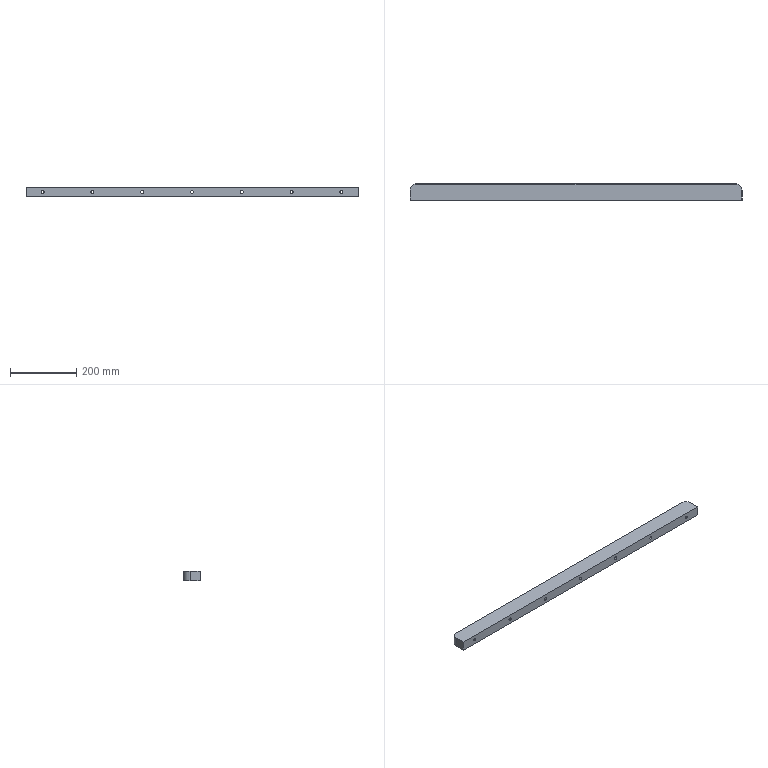Part | STEP file | TJ-DHQM-003-009 | 1 solid | 53 faces | box 1000 x 50 x 30 mm | volume 1451710 mm3 | cylinder 30 | plane 19 | cone 4 | commonest cylinder face diameters 9 x14 15 x14 40 x2
STEP:
#1=CARTESIAN_POINT('',(450.,25.,-7.5));
#2=VERTEX_POINT('',#1);
#3=CARTESIAN_POINT('',(450.,25.,7.5));
#4=VERTEX_POINT('',#3);
#5=CARTESIAN_POINT('',(450.,25.,0.));
#6=DIRECTION('',(0.,1.,0.));
#7=DIRECTION('',(0.,0.,1.));
#8=AXIS2_PLACEMENT_3D('',#5,#6,#7);
#9=CIRCLE('',#8,7.5);
#10=EDGE_CURVE('',#2,#4,#9,.T.);
#11=ORIENTED_EDGE('',*,*,#10,.F.);
#12=CARTESIAN_POINT('',(450.,50.,-7.5));
#13=VERTEX_POINT('',#12);
#14=CARTESIAN_POINT('',(450.,50.,-7.5));
#15=DIRECTION('',(0.,1.,0.));
#16=VECTOR('',#15,1000.);
#17=LINE('',#14,#16);
#18=EDGE_CURVE('',#2,#13,#17,.T.);
#19=ORIENTED_EDGE('',*,*,#18,.T.);
#20=CARTESIAN_POINT('',(450.,50.,7.5));
#21=VERTEX_POINT('',#20);
#22=CARTESIAN_POINT('',(450.,50.,0.));
#23=DIRECTION('',(0.,1.,0.));
#24=DIRECTION('',(0.,0.,1.));
#25=AXIS2_PLACEMENT_3D('',#22,#23,#24);
#26=CIRCLE('',#25,7.5);
#27=EDGE_CURVE('',#13,#21,#26,.T.);
#28=ORIENTED_EDGE('',*,*,#27,.T.);
#29=CARTESIAN_POINT('',(450.,50.,7.5));
#30=DIRECTION('',(0.,1.,0.));
#31=VECTOR('',#30,1000.);
#32=LINE('',#29,#31);
#33=EDGE_CURVE('',#4,#21,#32,.T.);
#34=ORIENTED_EDGE('',*,*,#33,.F.);
#35=EDGE_LOOP('',(#11,#19,#28,#34));
#36=FACE_OUTER_BOUND('',#35,.T.);
#37=CARTESIAN_POINT('',(450.,50.,0.));
#38=DIRECTION('',(0.,1.,0.));
#39=DIRECTION('',(0.,0.,1.));
#40=AXIS2_PLACEMENT_3D('',#37,#38,#39);
#41=CYLINDRICAL_SURFACE('',#40,7.5);
#42=ADVANCED_FACE('',(#36),#41,.F.);
#43=CARTESIAN_POINT('',(450.,0.,-4.5));
#44=VERTEX_POINT('',#43);
#45=CARTESIAN_POINT('',(450.,0.,4.5));
#46=VERTEX_POINT('',#45);
#47=CARTESIAN_POINT('',(450.,0.,0.));
#48=DIRECTION('',(0.,1.,0.));
#49=DIRECTION('',(0.,0.,1.));
#50=AXIS2_PLACEMENT_3D('',#47,#48,#49);
#51=CIRCLE('',#50,4.5);
#52=EDGE_CURVE('',#44,#46,#51,.T.);
#53=ORIENTED_EDGE('',*,*,#52,.F.);
#54=CARTESIAN_POINT('',(450.,25.,-4.5));
#55=VERTEX_POINT('',#54);
#56=CARTESIAN_POINT('',(450.,50.,-4.5));
#57=DIRECTION('',(0.,1.,0.));
#58=VECTOR('',#57,1000.);
#59=LINE('',#56,#58);
#60=EDGE_CURVE('',#44,#55,#59,.T.);
#61=ORIENTED_EDGE('',*,*,#60,.T.);
#62=CARTESIAN_POINT('',(450.,25.,4.5));
#63=VERTEX_POINT('',#62);
#64=CARTESIAN_POINT('',(450.,25.,0.));
#65=DIRECTION('',(0.,1.,0.));
#66=DIRECTION('',(0.,0.,1.));
#67=AXIS2_PLACEMENT_3D('',#64,#65,#66);
#68=CIRCLE('',#67,4.5);
#69=EDGE_CURVE('',#55,#63,#68,.T.);
#70=ORIENTED_EDGE('',*,*,#69,.T.);
#71=CARTESIAN_POINT('',(450.,50.,4.5));
#72=DIRECTION('',(0.,1.,0.));
#73=VECTOR('',#72,1000.);
#74=LINE('',#71,#73);
#75=EDGE_CURVE('',#46,#63,#74,.T.);
#76=ORIENTED_EDGE('',*,*,#75,.F.);
#77=EDGE_LOOP('',(#53,#61,#70,#76));
#78=FACE_OUTER_BOUND('',#77,.T.);
#79=CARTESIAN_POINT('',(450.,50.,0.));
#80=DIRECTION('',(0.,1.,0.));
#81=DIRECTION('',(0.,0.,1.));
#82=AXIS2_PLACEMENT_3D('',#79,#80,#81);
#83=CYLINDRICAL_SURFACE('',#82,4.5);
#84=ADVANCED_FACE('',(#78),#83,.F.);
#85=CARTESIAN_POINT('',(300.,25.,-7.5));
#86=VERTEX_POINT('',#85);
#87=CARTESIAN_POINT('',(300.,25.,7.5));
#88=VERTEX_POINT('',#87);
#89=CARTESIAN_POINT('',(300.,25.,0.));
#90=DIRECTION('',(0.,1.,0.));
#91=DIRECTION('',(0.,0.,1.));
#92=AXIS2_PLACEMENT_3D('',#89,#90,#91);
#93=CIRCLE('',#92,7.5);
#94=EDGE_CURVE('',#86,#88,#93,.T.);
#95=ORIENTED_EDGE('',*,*,#94,.F.);
#96=CARTESIAN_POINT('',(300.,50.,-7.5));
#97=VERTEX_POINT('',#96);
#98=CARTESIAN_POINT('',(300.,50.,-7.5));
#99=DIRECTION('',(0.,1.,0.));
#100=VECTOR('',#99,1000.);
#101=LINE('',#98,#100);
#102=EDGE_CURVE('',#86,#97,#101,.T.);
#103=ORIENTED_EDGE('',*,*,#102,.T.);
#104=CARTESIAN_POINT('',(300.,50.,7.5));
#105=VERTEX_POINT('',#104);
#106=CARTESIAN_POINT('',(300.,50.,0.));
#107=DIRECTION('',(0.,1.,0.));
#108=DIRECTION('',(0.,0.,1.));
#109=AXIS2_PLACEMENT_3D('',#106,#107,#108);
#110=CIRCLE('',#109,7.5);
#111=EDGE_CURVE('',#97,#105,#110,.T.);
#112=ORIENTED_EDGE('',*,*,#111,.T.);
#113=CARTESIAN_POINT('',(300.,50.,7.5));
#114=DIRECTION('',(0.,1.,0.));
#115=VECTOR('',#114,1000.);
#116=LINE('',#113,#115);
#117=EDGE_CURVE('',#88,#105,#116,.T.);
#118=ORIENTED_EDGE('',*,*,#117,.F.);
#119=EDGE_LOOP('',(#95,#103,#112,#118));
#120=FACE_OUTER_BOUND('',#119,.T.);
#121=CARTESIAN_POINT('',(300.,50.,0.));
#122=DIRECTION('',(0.,1.,0.));
#123=DIRECTION('',(0.,0.,1.));
#124=AXIS2_PLACEMENT_3D('',#121,#122,#123);
#125=CYLINDRICAL_SURFACE('',#124,7.5);
#126=ADVANCED_FACE('',(#120),#125,.F.);
#127=CARTESIAN_POINT('',(300.,0.,-4.5));
#128=VERTEX_POINT('',#127);
#129=CARTESIAN_POINT('',(300.,0.,4.5));
#130=VERTEX_POINT('',#129);
#131=CARTESIAN_POINT('',(300.,0.,0.));
#132=DIRECTION('',(0.,1.,0.));
#133=DIRECTION('',(0.,0.,1.));
#134=AXIS2_PLACEMENT_3D('',#131,#132,#133);
#135=CIRCLE('',#134,4.5);
#136=EDGE_CURVE('',#128,#130,#135,.T.);
#137=ORIENTED_EDGE('',*,*,#136,.F.);
#138=CARTESIAN_POINT('',(300.,25.,-4.5));
#139=VERTEX_POINT('',#138);
#140=CARTESIAN_POINT('',(300.,50.,-4.5));
#141=DIRECTION('',(0.,1.,0.));
#142=VECTOR('',#141,1000.);
#143=LINE('',#140,#142);
#144=EDGE_CURVE('',#128,#139,#143,.T.);
#145=ORIENTED_EDGE('',*,*,#144,.T.);
#146=CARTESIAN_POINT('',(300.,25.,4.5));
#147=VERTEX_POINT('',#146);
#148=CARTESIAN_POINT('',(300.,25.,0.));
#149=DIRECTION('',(0.,1.,0.));
#150=DIRECTION('',(0.,0.,1.));
#151=AXIS2_PLACEMENT_3D('',#148,#149,#150);
#152=CIRCLE('',#151,4.5);
#153=EDGE_CURVE('',#139,#147,#152,.T.);
#154=ORIENTED_EDGE('',*,*,#153,.T.);
#155=CARTESIAN_POINT('',(300.,50.,4.5));
#156=DIRECTION('',(0.,1.,0.));
#157=VECTOR('',#156,1000.);
#158=LINE('',#155,#157);
#159=EDGE_CURVE('',#130,#147,#158,.T.);
#160=ORIENTED_EDGE('',*,*,#159,.F.);
#161=EDGE_LOOP('',(#137,#145,#154,#160));
#162=FACE_OUTER_BOUND('',#161,.T.);
#163=CARTESIAN_POINT('',(300.,50.,0.));
#164=DIRECTION('',(0.,1.,0.));
#165=DIRECTION('',(0.,0.,1.));
#166=AXIS2_PLACEMENT_3D('',#163,#164,#165);
#167=CYLINDRICAL_SURFACE('',#166,4.5);
#168=ADVANCED_FACE('',(#162),#167,.F.);
#169=CARTESIAN_POINT('',(150.,25.,-7.5));
#170=VERTEX_POINT('',#169);
#171=CARTESIAN_POINT('',(150.,25.,7.5));
#172=VERTEX_POINT('',#171);
#173=CARTESIAN_POINT('',(150.,25.,0.));
#174=DIRECTION('',(0.,1.,0.));
#175=DIRECTION('',(0.,0.,1.));
#176=AXIS2_PLACEMENT_3D('',#173,#174,#175);
#177=CIRCLE('',#176,7.5);
#178=EDGE_CURVE('',#170,#172,#177,.T.);
#179=ORIENTED_EDGE('',*,*,#178,.F.);
#180=CARTESIAN_POINT('',(150.,50.,-7.5));
#181=VERTEX_POINT('',#180);
#182=CARTESIAN_POINT('',(150.,50.,-7.5));
#183=DIRECTION('',(0.,1.,0.));
#184=VECTOR('',#183,1000.);
#185=LINE('',#182,#184);
#186=EDGE_CURVE('',#170,#181,#185,.T.);
#187=ORIENTED_EDGE('',*,*,#186,.T.);
#188=CARTESIAN_POINT('',(150.,50.,7.5));
#189=VERTEX_POINT('',#188);
#190=CARTESIAN_POINT('',(150.,50.,0.));
#191=DIRECTION('',(0.,1.,0.));
#192=DIRECTION('',(0.,0.,1.));
#193=AXIS2_PLACEMENT_3D('',#190,#191,#192);
#194=CIRCLE('',#193,7.5);
#195=EDGE_CURVE('',#181,#189,#194,.T.);
#196=ORIENTED_EDGE('',*,*,#195,.T.);
#197=CARTESIAN_POINT('',(150.,50.,7.5));
#198=DIRECTION('',(0.,1.,0.));
#199=VECTOR('',#198,1000.);
#200=LINE('',#197,#199);
#201=EDGE_CURVE('',#172,#189,#200,.T.);
#202=ORIENTED_EDGE('',*,*,#201,.F.);
#203=EDGE_LOOP('',(#179,#187,#196,#202));
#204=FACE_OUTER_BOUND('',#203,.T.);
#205=CARTESIAN_POINT('',(150.,50.,0.));
#206=DIRECTION('',(0.,1.,0.));
#207=DIRECTION('',(0.,0.,1.));
#208=AXIS2_PLACEMENT_3D('',#205,#206,#207);
#209=CYLINDRICAL_SURFACE('',#208,7.5);
#210=ADVANCED_FACE('',(#204),#209,.F.);
#211=CARTESIAN_POINT('',(150.,0.,-4.5));
#212=VERTEX_POINT('',#211);
#213=CARTESIAN_POINT('',(150.,0.,4.5));
#214=VERTEX_POINT('',#213);
#215=CARTESIAN_POINT('',(150.,0.,0.));
#216=DIRECTION('',(0.,1.,0.));
#217=DIRECTION('',(0.,0.,1.));
#218=AXIS2_PLACEMENT_3D('',#215,#216,#217);
#219=CIRCLE('',#218,4.5);
#220=EDGE_CURVE('',#212,#214,#219,.T.);
#221=ORIENTED_EDGE('',*,*,#220,.F.);
#222=CARTESIAN_POINT('',(150.,25.,-4.5));
#223=VERTEX_POINT('',#222);
#224=CARTESIAN_POINT('',(150.,50.,-4.5));
#225=DIRECTION('',(0.,1.,0.));
#226=VECTOR('',#225,1000.);
#227=LINE('',#224,#226);
#228=EDGE_CURVE('',#212,#223,#227,.T.);
#229=ORIENTED_EDGE('',*,*,#228,.T.);
#230=CARTESIAN_POINT('',(150.,25.,4.5));
#231=VERTEX_POINT('',#230);
#232=CARTESIAN_POINT('',(150.,25.,0.));
#233=DIRECTION('',(0.,1.,0.));
#234=DIRECTION('',(0.,0.,1.));
#235=AXIS2_PLACEMENT_3D('',#232,#233,#234);
#236=CIRCLE('',#235,4.5);
#237=EDGE_CURVE('',#223,#231,#236,.T.);
#238=ORIENTED_EDGE('',*,*,#237,.T.);
#239=CARTESIAN_POINT('',(150.,50.,4.5));
#240=DIRECTION('',(0.,1.,0.));
#241=VECTOR('',#240,1000.);
#242=LINE('',#239,#241);
#243=EDGE_CURVE('',#214,#231,#242,.T.);
#244=ORIENTED_EDGE('',*,*,#243,.F.);
#245=EDGE_LOOP('',(#221,#229,#238,#244));
#246=FACE_OUTER_BOUND('',#245,.T.);
#247=CARTESIAN_POINT('',(150.,50.,0.));
#248=DIRECTION('',(0.,1.,0.));
#249=DIRECTION('',(0.,0.,1.));
#250=AXIS2_PLACEMENT_3D('',#247,#248,#249);
#251=CYLINDRICAL_SURFACE('',#250,4.5);
#252=ADVANCED_FACE('',(#246),#251,.F.);
#253=CARTESIAN_POINT('',(-450.,25.,-7.5));
#254=VERTEX_POINT('',#253);
#255=CARTESIAN_POINT('',(-450.,25.,7.5));
#256=VERTEX_POINT('',#255);
#257=CARTESIAN_POINT('',(-450.,25.,0.));
#258=DIRECTION('',(0.,1.,0.));
#259=DIRECTION('',(0.,0.,1.));
#260=AXIS2_PLACEMENT_3D('',#257,#258,#259);
#261=CIRCLE('',#260,7.5);
#262=EDGE_CURVE('',#254,#256,#261,.T.);
#263=ORIENTED_EDGE('',*,*,#262,.F.);
#264=CARTESIAN_POINT('',(-450.,50.,-7.5));
#265=VERTEX_POINT('',#264);
#266=CARTESIAN_POINT('',(-450.,50.,-7.5));
#267=DIRECTION('',(0.,1.,0.));
#268=VECTOR('',#267,1000.);
#269=LINE('',#266,#268);
#270=EDGE_CURVE('',#254,#265,#269,.T.);
#271=ORIENTED_EDGE('',*,*,#270,.T.);
#272=CARTESIAN_POINT('',(-450.,50.,7.5));
#273=VERTEX_POINT('',#272);
#274=CARTESIAN_POINT('',(-450.,50.,0.));
#275=DIRECTION('',(0.,1.,0.));
#276=DIRECTION('',(0.,0.,1.));
#277=AXIS2_PLACEMENT_3D('',#274,#275,#276);
#278=CIRCLE('',#277,7.5);
#279=EDGE_CURVE('',#265,#273,#278,.T.);
#280=ORIENTED_EDGE('',*,*,#279,.T.);
#281=CARTESIAN_POINT('',(-450.,50.,7.5));
#282=DIRECTION('',(0.,1.,0.));
#283=VECTOR('',#282,1000.);
#284=LINE('',#281,#283);
#285=EDGE_CURVE('',#256,#273,#284,.T.);
#286=ORIENTED_EDGE('',*,*,#285,.F.);
#287=EDGE_LOOP('',(#263,#271,#280,#286));
#288=FACE_OUTER_BOUND('',#287,.T.);
#289=CARTESIAN_POINT('',(-450.,50.,0.));
#290=DIRECTION('',(0.,1.,0.));
#291=DIRECTION('',(0.,0.,1.));
#292=AXIS2_PLACEMENT_3D('',#289,#290,#291);
#293=CYLINDRICAL_SURFACE('',#292,7.5);
#294=ADVANCED_FACE('',(#288),#293,.F.);
#295=CARTESIAN_POINT('',(-450.,0.,-4.5));
#296=VERTEX_POINT('',#295);
#297=CARTESIAN_POINT('',(-450.,0.,4.5));
#298=VERTEX_POINT('',#297);
#299=CARTESIAN_POINT('',(-450.,0.,0.));
#300=DIRECTION('',(0.,1.,0.));
#301=DIRECTION('',(0.,0.,1.));
#302=AXIS2_PLACEMENT_3D('',#299,#300,#301);
#303=CIRCLE('',#302,4.5);
#304=EDGE_CURVE('',#296,#298,#303,.T.);
#305=ORIENTED_EDGE('',*,*,#304,.F.);
#306=CARTESIAN_POINT('',(-450.,25.,-4.5));
#307=VERTEX_POINT('',#306);
#308=CARTESIAN_POINT('',(-450.,50.,-4.5));
#309=DIRECTION('',(0.,1.,0.));
#310=VECTOR('',#309,1000.);
#311=LINE('',#308,#310);
#312=EDGE_CURVE('',#296,#307,#311,.T.);
#313=ORIENTED_EDGE('',*,*,#312,.T.);
#314=CARTESIAN_POINT('',(-450.,25.,4.5));
#315=VERTEX_POINT('',#314);
#316=CARTESIAN_POINT('',(-450.,25.,0.));
#317=DIRECTION('',(0.,1.,0.));
#318=DIRECTION('',(0.,0.,1.));
#319=AXIS2_PLACEMENT_3D('',#316,#317,#318);
#320=CIRCLE('',#319,4.5);
#321=EDGE_CURVE('',#307,#315,#320,.T.);
#322=ORIENTED_EDGE('',*,*,#321,.T.);
#323=CARTESIAN_POINT('',(-450.,50.,4.5));
#324=DIRECTION('',(0.,1.,0.));
#325=VECTOR('',#324,1000.);
#326=LINE('',#323,#325);
#327=EDGE_CURVE('',#298,#315,#326,.T.);
#328=ORIENTED_EDGE('',*,*,#327,.F.);
#329=EDGE_LOOP('',(#305,#313,#322,#328));
#330=FACE_OUTER_BOUND('',#329,.T.);
#331=CARTESIAN_POINT('',(-450.,50.,0.));
#332=DIRECTION('',(0.,1.,0.));
#333=DIRECTION('',(0.,0.,1.));
#334=AXIS2_PLACEMENT_3D('',#331,#332,#333);
#335=CYLINDRICAL_SURFACE('',#334,4.5);
#336=ADVANCED_FACE('',(#330),#335,.F.);
#337=CARTESIAN_POINT('',(-300.,25.,-7.5));
#338=VERTEX_POINT('',#337);
#339=CARTESIAN_POINT('',(-300.,25.,7.5));
#340=VERTEX_POINT('',#339);
#341=CARTESIAN_POINT('',(-300.,25.,0.));
#342=DIRECTION('',(0.,1.,0.));
#343=DIRECTION('',(0.,0.,1.));
#344=AXIS2_PLACEMENT_3D('',#341,#342,#343);
#345=CIRCLE('',#344,7.5);
#346=EDGE_CURVE('',#338,#340,#345,.T.);
#347=ORIENTED_EDGE('',*,*,#346,.F.);
#348=CARTESIAN_POINT('',(-300.,50.,-7.5));
#349=VERTEX_POINT('',#348);
#350=CARTESIAN_POINT('',(-300.,50.,-7.5));
#351=DIRECTION('',(0.,1.,0.));
#352=VECTOR('',#351,1000.);
#353=LINE('',#350,#352);
#354=EDGE_CURVE('',#338,#349,#353,.T.);
#355=ORIENTED_EDGE('',*,*,#354,.T.);
#356=CARTESIAN_POINT('',(-300.,50.,7.5));
#357=VERTEX_POINT('',#356);
#358=CARTESIAN_POINT('',(-300.,50.,0.));
#359=DIRECTION('',(0.,1.,0.));
#360=DIRECTION('',(0.,0.,1.));
#361=AXIS2_PLACEMENT_3D('',#358,#359,#360);
#362=CIRCLE('',#361,7.5);
#363=EDGE_CURVE('',#349,#357,#362,.T.);
#364=ORIENTED_EDGE('',*,*,#363,.T.);
#365=CARTESIAN_POINT('',(-300.,50.,7.5));
#366=DIRECTION('',(0.,1.,0.));
#367=VECTOR('',#366,1000.);
#368=LINE('',#365,#367);
#369=EDGE_CURVE('',#340,#357,#368,.T.);
#370=ORIENTED_EDGE('',*,*,#369,.F.);
#371=EDGE_LOOP('',(#347,#355,#364,#370));
#372=FACE_OUTER_BOUND('',#371,.T.);
#373=CARTESIAN_POINT('',(-300.,50.,0.));
#374=DIRECTION('',(0.,1.,0.));
#375=DIRECTION('',(0.,0.,1.));
#376=AXIS2_PLACEMENT_3D('',#373,#374,#375);
#377=CYLINDRICAL_SURFACE('',#376,7.5);
#378=ADVANCED_FACE('',(#372),#377,.F.);
#379=CARTESIAN_POINT('',(-300.,0.,-4.5));
#380=VERTEX_POINT('',#379);
#381=CARTESIAN_POINT('',(-300.,0.,4.5));
#382=VERTEX_POINT('',#381);
#383=CARTESIAN_POINT('',(-300.,0.,0.));
#384=DIRECTION('',(0.,1.,0.));
#385=DIRECTION('',(0.,0.,1.));
#386=AXIS2_PLACEMENT_3D('',#383,#384,#385);
#387=CIRCLE('',#386,4.5);
#388=EDGE_CURVE('',#380,#382,#387,.T.);
#389=ORIENTED_EDGE('',*,*,#388,.F.);
#390=CARTESIAN_POINT('',(-300.,25.,-4.5));
#391=VERTEX_POINT('',#390);
#392=CARTESIAN_POINT('',(-300.,50.,-4.5));
#393=DIRECTION('',(0.,1.,0.));
#394=VECTOR('',#393,1000.);
#395=LINE('',#392,#394);
#396=EDGE_CURVE('',#380,#391,#395,.T.);
#397=ORIENTED_EDGE('',*,*,#396,.T.);
#398=CARTESIAN_POINT('',(-300.,25.,4.5));
#399=VERTEX_POINT('',#398);
#400=CARTESIAN_POINT('',(-300.,25.,0.));
#401=DIRECTION('',(0.,1.,0.));
#402=DIRECTION('',(0.,0.,1.));
#403=AXIS2_PLACEMENT_3D('',#400,#401,#402);
#404=CIRCLE('',#403,4.5);
#405=EDGE_CURVE('',#391,#399,#404,.T.);
#406=ORIENTED_EDGE('',*,*,#405,.T.);
#407=CARTESIAN_POINT('',(-300.,50.,4.5));
#408=DIRECTION('',(0.,1.,0.));
#409=VECTOR('',#408,1000.);
#410=LINE('',#407,#409);
#411=EDGE_CURVE('',#382,#399,#410,.T.);
#412=ORIENTED_EDGE('',*,*,#411,.F.);
#413=EDGE_LOOP('',(#389,#397,#406,#412));
#414=FACE_OUTER_BOUND('',#413,.T.);
#415=CARTESIAN_POINT('',(-300.,50.,0.));
#416=DIRECTION('',(0.,1.,0.));
#417=DIRECTION('',(0.,0.,1.));
#418=AXIS2_PLACEMENT_3D('',#415,#416,#417);
#419=CYLINDRICAL_SURFACE('',#418,4.5);
#420=ADVANCED_FACE('',(#414),#419,.F.);
#421=CARTESIAN_POINT('',(-150.,25.,-7.5));
#422=VERTEX_POINT('',#421);
#423=CARTESIAN_POINT('',(-150.,25.,7.5));
#424=VERTEX_POINT('',#423);
#425=CARTESIAN_POINT('',(-150.,25.,0.));
#426=DIRECTION('',(0.,1.,0.));
#427=DIRECTION('',(0.,0.,1.));
#428=AXIS2_PLACEMENT_3D('',#425,#426,#427);
#429=CIRCLE('',#428,7.5);
#430=EDGE_CURVE('',#422,#424,#429,.T.);
#431=ORIENTED_EDGE('',*,*,#430,.F.);
#432=CARTESIAN_POINT('',(-150.,50.,-7.5));
#433=VERTEX_POINT('',#432);
#434=CARTESIAN_POINT('',(-150.,50.,-7.5));
#435=DIRECTION('',(0.,1.,0.));
#436=VECTOR('',#435,1000.);
#437=LINE('',#434,#436);
#438=EDGE_CURVE('',#422,#433,#437,.T.);
#439=ORIENTED_EDGE('',*,*,#438,.T.);
#440=CARTESIAN_POINT('',(-150.,50.,7.5));
#441=VERTEX_POINT('',#440);
#442=CARTESIAN_POINT('',(-150.,50.,0.));
#443=DIRECTION('',(0.,1.,0.));
#444=DIRECTION('',(0.,0.,1.));
#445=AXIS2_PLACEMENT_3D('',#442,#443,#444);
#446=CIRCLE('',#445,7.5);
#447=EDGE_CURVE('',#433,#441,#446,.T.);
#448=ORIENTED_EDGE('',*,*,#447,.T.);
#449=CARTESIAN_POINT('',(-150.,50.,7.5));
#450=DIRECTION('',(0.,1.,0.));
#451=VECTOR('',#450,1000.);
#452=LINE('',#449,#451);
#453=EDGE_CURVE('',#424,#441,#452,.T.);
#454=ORIENTED_EDGE('',*,*,#453,.F.);
#455=EDGE_LOOP('',(#431,#439,#448,#454));
#456=FACE_OUTER_BOUND('',#455,.T.);
#457=CARTESIAN_POINT('',(-150.,50.,0.));
#458=DIRECTION('',(0.,1.,0.));
#459=DIRECTION('',(0.,0.,1.));
#460=AXIS2_PLACEMENT_3D('',#457,#458,#459);
#461=CYLINDRICAL_SURFACE('',#460,7.5);
#462=ADVANCED_FACE('',(#456),#461,.F.);
#463=CARTESIAN_POINT('',(-150.,0.,-4.5));
#464=VERTEX_POINT('',#463);
#465=CARTESIAN_POINT('',(-150.,0.,4.5));
#466=VERTEX_POINT('',#465);
#467=CARTESIAN_POINT('',(-150.,0.,0.));
#468=DIRECTION('',(0.,1.,0.));
#469=DIRECTION('',(0.,0.,1.));
#470=AXIS2_PLACEMENT_3D('',#467,#468,#469);
#471=CIRCLE('',#470,4.5);
#472=EDGE_CURVE('',#464,#466,#471,.T.);
#473=ORIENTED_EDGE('',*,*,#472,.F.);
#474=CARTESIAN_POINT('',(-150.,25.,-4.5));
#475=VERTEX_POINT('',#474);
#476=CARTESIAN_POINT('',(-150.,50.,-4.5));
#477=DIRECTION('',(0.,1.,0.));
#478=VECTOR('',#477,1000.);
#479=LINE('',#476,#478);
#480=EDGE_CURVE('',#464,#475,#479,.T.);
#481=ORIENTED_EDGE('',*,*,#480,.T.);
#482=CARTESIAN_POINT('',(-150.,25.,4.5));
#483=VERTEX_POINT('',#482);
#484=CARTESIAN_POINT('',(-150.,25.,0.));
#485=DIRECTION('',(0.,1.,0.));
#486=DIRECTION('',(0.,0.,1.));
#487=AXIS2_PLACEMENT_3D('',#484,#485,#486);
#488=CIRCLE('',#487,4.5);
#489=EDGE_CURVE('',#475,#483,#488,.T.);
#490=ORIENTED_EDGE('',*,*,#489,.T.);
#491=CARTESIAN_POINT('',(-150.,50.,4.5));
#492=DIRECTION('',(0.,1.,0.));
#493=VECTOR('',#492,1000.);
#494=LINE('',#491,#493);
#495=EDGE_CURVE('',#466,#483,#494,.T.);
#496=ORIENTED_EDGE('',*,*,#495,.F.);
#497=EDGE_LOOP('',(#473,#481,#490,#496));
#498=FACE_OUTER_BOUND('',#497,.T.);
#499=CARTESIAN_POINT('',(-150.,50.,0.));
#500=DIRECTION('',(0.,1.,0.));
#501=DIRECTION('',(0.,0.,1.));
#502=AXIS2_PLACEMENT_3D('',#499,#500,#501);
#503=CYLINDRICAL_SURFACE('',#502,4.5);
#504=ADVANCED_FACE('',(#498),#503,.F.);
#505=CARTESIAN_POINT('',(0.,25.,-7.5));
#506=VERTEX_POINT('',#505);
#507=CARTESIAN_POINT('',(0.,25.,7.5));
#508=VERTEX_POINT('',#507);
#509=CARTESIAN_POINT('',(0.,25.,0.));
#510=DIRECTION('',(0.,1.,0.));
#511=DIRECTION('',(0.,0.,1.));
#512=AXIS2_PLACEMENT_3D('',#509,#510,#511);
#513=CIRCLE('',#512,7.5);
#514=EDGE_CURVE('',#506,#508,#513,.T.);
#515=ORIENTED_EDGE('',*,*,#514,.F.);
#516=CARTESIAN_POINT('',(0.,50.,-7.5));
#517=VERTEX_POINT('',#516);
#518=CARTESIAN_POINT('',(0.,50.,-7.5));
#519=DIRECTION('',(0.,1.,0.));
#520=VECTOR('',#519,1000.);
#521=LINE('',#518,#520);
#522=EDGE_CURVE('',#506,#517,#521,.T.);
#523=ORIENTED_EDGE('',*,*,#522,.T.);
#524=CARTESIAN_POINT('',(0.,50.,7.5));
#525=VERTEX_POINT('',#524);
#526=CARTESIAN_POINT('',(0.,50.,0.));
#527=DIRECTION('',(0.,1.,0.));
#528=DIRECTION('',(0.,0.,1.));
#529=AXIS2_PLACEMENT_3D('',#526,#527,#528);
#530=CIRCLE('',#529,7.5);
#531=EDGE_CURVE('',#517,#525,#530,.T.);
#532=ORIENTED_EDGE('',*,*,#531,.T.);
#533=CARTESIAN_POINT('',(0.,50.,7.5));
#534=DIRECTION('',(0.,1.,0.));
#535=VECTOR('',#534,1000.);
#536=LINE('',#533,#535);
#537=EDGE_CURVE('',#508,#525,#536,.T.);
#538=ORIENTED_EDGE('',*,*,#537,.F.);
#539=EDGE_LOOP('',(#515,#523,#532,#538));
#540=FACE_OUTER_BOUND('',#539,.T.);
#541=CARTESIAN_POINT('',(0.,50.,0.));
#542=DIRECTION('',(0.,1.,0.));
#543=DIRECTION('',(0.,0.,1.));
#544=AXIS2_PLACEMENT_3D('',#541,#542,#543);
#545=CYLINDRICAL_SURFACE('',#544,7.5);
#546=ADVANCED_FACE('',(#540),#545,.F.);
#547=CARTESIAN_POINT('',(0.,0.,-4.5));
#548=VERTEX_POINT('',#547);
#549=CARTESIAN_POINT('',(0.,0.,4.5));
#550=VERTEX_POINT('',#549);
#551=CARTESIAN_POINT('',(0.,0.,0.));
#552=DIRECTION('',(0.,1.,0.));
#553=DIRECTION('',(0.,0.,1.));
#554=AXIS2_PLACEMENT_3D('',#551,#552,#553);
#555=CIRCLE('',#554,4.5);
#556=EDGE_CURVE('',#548,#550,#555,.T.);
#557=ORIENTED_EDGE('',*,*,#556,.F.);
#558=CARTESIAN_POINT('',(0.,25.,-4.5));
#559=VERTEX_POINT('',#558);
#560=CARTESIAN_POINT('',(0.,50.,-4.5));
#561=DIRECTION('',(0.,1.,0.));
#562=VECTOR('',#561,1000.);
#563=LINE('',#560,#562);
#564=EDGE_CURVE('',#548,#559,#563,.T.);
#565=ORIENTED_EDGE('',*,*,#564,.T.);
#566=CARTESIAN_POINT('',(0.,25.,4.5));
#567=VERTEX_POINT('',#566);
#568=CARTESIAN_POINT('',(0.,25.,0.));
#569=DIRECTION('',(0.,1.,0.));
#570=DIRECTION('',(0.,0.,1.));
#571=AXIS2_PLACEMENT_3D('',#568,#569,#570);
#572=CIRCLE('',#571,4.5);
#573=EDGE_CURVE('',#559,#567,#572,.T.);
#574=ORIENTED_EDGE('',*,*,#573,.T.);
#575=CARTESIAN_POINT('',(0.,50.,4.5));
#576=DIRECTION('',(0.,1.,0.));
#577=VECTOR('',#576,1000.);
#578=LINE('',#575,#577);
#579=EDGE_CURVE('',#550,#567,#578,.T.);
#580=ORIENTED_EDGE('',*,*,#579,.F.);
#581=EDGE_LOOP('',(#557,#565,#574,#580));
#582=FACE_OUTER_BOUND('',#581,.T.);
#583=CARTESIAN_POINT('',(0.,50.,0.));
#584=DIRECTION('',(0.,1.,0.));
#585=DIRECTION('',(0.,0.,1.));
#586=AXIS2_PLACEMENT_3D('',#583,#584,#585);
#587=CYLINDRICAL_SURFACE('',#586,4.5);
#588=ADVANCED_FACE('',(#582),#587,.F.);
#589=CARTESIAN_POINT('',(-500.,30.,14.));
#590=VERTEX_POINT('',#589);
#591=CARTESIAN_POINT('',(-500.,30.,-14.));
#592=VERTEX_POINT('',#591);
#593=CARTESIAN_POINT('',(-500.,30.,-15.));
#594=DIRECTION('',(0.,0.,-1.));
#595=VECTOR('',#594,1000.);
#596=LINE('',#593,#595);
#597=EDGE_CURVE('',#590,#592,#596,.T.);
#598=ORIENTED_EDGE('',*,*,#597,.T.);
#599=CARTESIAN_POINT('',(-500.,0.,-14.));
#600=VERTEX_POINT('',#599);
#601=CARTESIAN_POINT('',(-500.,0.,-14.));
#602=DIRECTION('',(0.,-1.,0.));
#603=VECTOR('',#602,1000.);
#604=LINE('',#601,#603);
#605=EDGE_CURVE('',#592,#600,#604,.T.);
#606=ORIENTED_EDGE('',*,*,#605,.T.);
#607=CARTESIAN_POINT('',(-500.,0.,14.));
#608=VERTEX_POINT('',#607);
#609=CARTESIAN_POINT('',(-500.,0.,-15.));
#610=DIRECTION('',(0.,0.,1.));
#611=VECTOR('',#610,1000.);
#612=LINE('',#609,#611);
#613=EDGE_CURVE('',#600,#608,#612,.T.);
#614=ORIENTED_EDGE('',*,*,#613,.T.);
#615=CARTESIAN_POINT('',(-500.,30.,14.));
#616=DIRECTION('',(0.,1.,0.));
#617=VECTOR('',#616,1000.);
#618=LINE('',#615,#617);
#619=EDGE_CURVE('',#608,#590,#618,.T.);
#620=ORIENTED_EDGE('',*,*,#619,.T.);
#621=EDGE_LOOP('',(#598,#606,#614,#620));
#622=FACE_OUTER_BOUND('',#621,.T.);
#623=CARTESIAN_POINT('',(-500.,0.,-15.));
#624=DIRECTION('',(-1.,0.,0.));
#625=DIRECTION('',(0.,0.,1.));
#626=AXIS2_PLACEMENT_3D('',#623,#624,#625);
#627=PLANE('',#626);
#628=ADVANCED_FACE('',(#622),#627,.T.);
#629=CARTESIAN_POINT('',(450.,50.,0.));
#630=DIRECTION('',(0.,1.,0.));
#631=DIRECTION('',(0.,0.,1.));
#632=AXIS2_PLACEMENT_3D('',#629,#630,#631);
#633=CIRCLE('',#632,7.5);
#634=EDGE_CURVE('',#21,#13,#633,.T.);
#635=ORIENTED_EDGE('',*,*,#634,.F.);
#636=ORIENTED_EDGE('',*,*,#27,.F.);
#637=EDGE_LOOP('',(#635,#636));
#638=FACE_BOUND('',#637,.T.);
#639=CARTESIAN_POINT('',(300.,50.,0.));
#640=DIRECTION('',(0.,1.,0.));
#641=DIRECTION('',(0.,0.,1.));
#642=AXIS2_PLACEMENT_3D('',#639,#640,#641);
#643=CIRCLE('',#642,7.5);
#644=EDGE_CURVE('',#105,#97,#643,.T.);
#645=ORIENTED_EDGE('',*,*,#644,.F.);
#646=ORIENTED_EDGE('',*,*,#111,.F.);
#647=EDGE_LOOP('',(#645,#646));
#648=FACE_BOUND('',#647,.T.);
#649=CARTESIAN_POINT('',(150.,50.,0.));
#650=DIRECTION('',(0.,1.,0.));
#651=DIRECTION('',(0.,0.,1.));
#652=AXIS2_PLACEMENT_3D('',#649,#650,#651);
#653=CIRCLE('',#652,7.5);
#654=EDGE_CURVE('',#189,#181,#653,.T.);
#655=ORIENTED_EDGE('',*,*,#654,.F.);
#656=ORIENTED_EDGE('',*,*,#195,.F.);
#657=EDGE_LOOP('',(#655,#656));
#658=FACE_BOUND('',#657,.T.);
#659=CARTESIAN_POINT('',(-450.,50.,0.));
#660=DIRECTION('',(0.,1.,0.));
#661=DIRECTION('',(0.,0.,1.));
#662=AXIS2_PLACEMENT_3D('',#659,#660,#661);
#663=CIRCLE('',#662,7.5);
#664=EDGE_CURVE('',#273,#265,#663,.T.);
#665=ORIENTED_EDGE('',*,*,#664,.F.);
#666=ORIENTED_EDGE('',*,*,#279,.F.);
#667=EDGE_LOOP('',(#665,#666));
#668=FACE_BOUND('',#667,.T.);
#669=CARTESIAN_POINT('',(-300.,50.,0.));
#670=DIRECTION('',(0.,1.,0.));
#671=DIRECTION('',(0.,0.,1.));
#672=AXIS2_PLACEMENT_3D('',#669,#670,#671);
#673=CIRCLE('',#672,7.5);
#674=EDGE_CURVE('',#357,#349,#673,.T.);
#675=ORIENTED_EDGE('',*,*,#674,.F.);
#676=ORIENTED_EDGE('',*,*,#363,.F.);
#677=EDGE_LOOP('',(#675,#676));
#678=FACE_BOUND('',#677,.T.);
#679=CARTESIAN_POINT('',(-150.,50.,0.));
#680=DIRECTION('',(0.,1.,0.));
#681=DIRECTION('',(0.,0.,1.));
#682=AXIS2_PLACEMENT_3D('',#679,#680,#681);
#683=CIRCLE('',#682,7.5);
#684=EDGE_CURVE('',#441,#433,#683,.T.);
#685=ORIENTED_EDGE('',*,*,#684,.F.);
#686=ORIENTED_EDGE('',*,*,#447,.F.);
#687=EDGE_LOOP('',(#685,#686));
#688=FACE_BOUND('',#687,.T.);
#689=CARTESIAN_POINT('',(0.,50.,0.));
#690=DIRECTION('',(0.,1.,0.));
#691=DIRECTION('',(0.,0.,1.));
#692=AXIS2_PLACEMENT_3D('',#689,#690,#691);
#693=CIRCLE('',#692,7.5);
#694=EDGE_CURVE('',#525,#517,#693,.T.);
#695=ORIENTED_EDGE('',*,*,#694,.F.);
#696=ORIENTED_EDGE('',*,*,#531,.F.);
#697=EDGE_LOOP('',(#695,#696));
#698=FACE_BOUND('',#697,.T.);
#699=CARTESIAN_POINT('',(480.,50.,14.));
#700=VERTEX_POINT('',#699);
#701=CARTESIAN_POINT('',(480.,50.,-14.));
#702=VERTEX_POINT('',#701);
#703=CARTESIAN_POINT('',(480.,50.,-15.));
#704=DIRECTION('',(0.,0.,-1.));
#705=VECTOR('',#704,1000.);
#706=LINE('',#703,#705);
#707=EDGE_CURVE('',#700,#702,#706,.T.);
#708=ORIENTED_EDGE('',*,*,#707,.T.);
#709=CARTESIAN_POINT('',(-480.,50.,-14.));
#710=VERTEX_POINT('',#709);
#711=CARTESIAN_POINT('',(-500.,50.,-14.));
#712=DIRECTION('',(-1.,0.,0.));
#713=VECTOR('',#712,1000.);
#714=LINE('',#711,#713);
#715=EDGE_CURVE('',#702,#710,#714,.T.);
#716=ORIENTED_EDGE('',*,*,#715,.T.);
#717=CARTESIAN_POINT('',(-480.,50.,14.));
#718=VERTEX_POINT('',#717);
#719=CARTESIAN_POINT('',(-480.,50.,-15.));
#720=DIRECTION('',(0.,0.,1.));
#721=VECTOR('',#720,1000.);
#722=LINE('',#719,#721);
#723=EDGE_CURVE('',#710,#718,#722,.T.);
#724=ORIENTED_EDGE('',*,*,#723,.T.);
#725=CARTESIAN_POINT('',(480.,50.,14.));
#726=DIRECTION('',(1.,0.,0.));
#727=VECTOR('',#726,1000.);
#728=LINE('',#725,#727);
#729=EDGE_CURVE('',#718,#700,#728,.T.);
#730=ORIENTED_EDGE('',*,*,#729,.T.);
#731=EDGE_LOOP('',(#708,#716,#724,#730));
#732=FACE_OUTER_BOUND('',#731,.T.);
#733=CARTESIAN_POINT('',(-500.,50.,-15.));
#734=DIRECTION('',(0.,1.,0.));
#735=DIRECTION('',(0.,0.,1.));
#736=AXIS2_PLACEMENT_3D('',#733,#734,#735);
#737=PLANE('',#736);
#738=ADVANCED_FACE('',(#638,#648,#658,#668,#678,#688,#698,#732),#737,.T.);
#739=CARTESIAN_POINT('',(500.,0.,-14.));
#740=VERTEX_POINT('',#739);
#741=CARTESIAN_POINT('',(500.,0.,14.));
#742=VERTEX_POINT('',#741);
#743=CARTESIAN_POINT('',(500.,0.,-15.));
#744=DIRECTION('',(0.,0.,1.));
#745=VECTOR('',#744,1000.);
#746=LINE('',#743,#745);
#747=EDGE_CURVE('',#740,#742,#746,.T.);
#748=ORIENTED_EDGE('',*,*,#747,.F.);
#749=CARTESIAN_POINT('',(500.,30.,-14.));
#750=VERTEX_POINT('',#749);
#751=CARTESIAN_POINT('',(500.,0.,-14.));
#752=DIRECTION('',(0.,1.,0.));
#753=VECTOR('',#752,1000.);
#754=LINE('',#751,#753);
#755=EDGE_CURVE('',#740,#750,#754,.T.);
#756=ORIENTED_EDGE('',*,*,#755,.T.);
#757=CARTESIAN_POINT('',(500.,30.,14.));
#758=VERTEX_POINT('',#757);
#759=CARTESIAN_POINT('',(500.,30.,-15.));
#760=DIRECTION('',(0.,0.,1.));
#761=VECTOR('',#760,1000.);
#762=LINE('',#759,#761);
#763=EDGE_CURVE('',#750,#758,#762,.T.);
#764=ORIENTED_EDGE('',*,*,#763,.T.);
#765=CARTESIAN_POINT('',(500.,0.,14.));
#766=DIRECTION('',(0.,-1.,0.));
#767=VECTOR('',#766,1000.);
#768=LINE('',#765,#767);
#769=EDGE_CURVE('',#758,#742,#768,.T.);
#770=ORIENTED_EDGE('',*,*,#769,.T.);
#771=EDGE_LOOP('',(#748,#756,#764,#770));
#772=FACE_OUTER_BOUND('',#771,.T.);
#773=CARTESIAN_POINT('',(500.,0.,-15.));
#774=DIRECTION('',(1.,0.,0.));
#775=DIRECTION('',(0.,0.,-1.));
#776=AXIS2_PLACEMENT_3D('',#773,#774,#775);
#777=PLANE('',#776);
#778=ADVANCED_FACE('',(#772),#777,.T.);
#779=CARTESIAN_POINT('',(450.,0.,0.));
#780=DIRECTION('',(0.,1.,0.));
#781=DIRECTION('',(0.,0.,1.));
#782=AXIS2_PLACEMENT_3D('',#779,#780,#781);
#783=CIRCLE('',#782,4.5);
#784=EDGE_CURVE('',#46,#44,#783,.T.);
#785=ORIENTED_EDGE('',*,*,#784,.T.);
#786=ORIENTED_EDGE('',*,*,#52,.T.);
#787=EDGE_LOOP('',(#785,#786));
#788=FACE_BOUND('',#787,.T.);
#789=CARTESIAN_POINT('',(300.,0.,0.));
#790=DIRECTION('',(0.,1.,0.));
#791=DIRECTION('',(0.,0.,1.));
#792=AXIS2_PLACEMENT_3D('',#789,#790,#791);
#793=CIRCLE('',#792,4.5);
#794=EDGE_CURVE('',#130,#128,#793,.T.);
#795=ORIENTED_EDGE('',*,*,#794,.T.);
#796=ORIENTED_EDGE('',*,*,#136,.T.);
#797=EDGE_LOOP('',(#795,#796));
#798=FACE_BOUND('',#797,.T.);
#799=CARTESIAN_POINT('',(150.,0.,0.));
#800=DIRECTION('',(0.,1.,0.));
#801=DIRECTION('',(0.,0.,1.));
#802=AXIS2_PLACEMENT_3D('',#799,#800,#801);
#803=CIRCLE('',#802,4.5);
#804=EDGE_CURVE('',#214,#212,#803,.T.);
#805=ORIENTED_EDGE('',*,*,#804,.T.);
#806=ORIENTED_EDGE('',*,*,#220,.T.);
#807=EDGE_LOOP('',(#805,#806));
#808=FACE_BOUND('',#807,.T.);
#809=CARTESIAN_POINT('',(-450.,0.,0.));
#810=DIRECTION('',(0.,1.,0.));
#811=DIRECTION('',(0.,0.,1.));
#812=AXIS2_PLACEMENT_3D('',#809,#810,#811);
#813=CIRCLE('',#812,4.5);
#814=EDGE_CURVE('',#298,#296,#813,.T.);
#815=ORIENTED_EDGE('',*,*,#814,.T.);
#816=ORIENTED_EDGE('',*,*,#304,.T.);
#817=EDGE_LOOP('',(#815,#816));
#818=FACE_BOUND('',#817,.T.);
#819=CARTESIAN_POINT('',(-300.,0.,0.));
#820=DIRECTION('',(0.,1.,0.));
#821=DIRECTION('',(0.,0.,1.));
#822=AXIS2_PLACEMENT_3D('',#819,#820,#821);
#823=CIRCLE('',#822,4.5);
#824=EDGE_CURVE('',#382,#380,#823,.T.);
#825=ORIENTED_EDGE('',*,*,#824,.T.);
#826=ORIENTED_EDGE('',*,*,#388,.T.);
#827=EDGE_LOOP('',(#825,#826));
#828=FACE_BOUND('',#827,.T.);
#829=CARTESIAN_POINT('',(-150.,0.,0.));
#830=DIRECTION('',(0.,1.,0.));
#831=DIRECTION('',(0.,0.,1.));
#832=AXIS2_PLACEMENT_3D('',#829,#830,#831);
#833=CIRCLE('',#832,4.5);
#834=EDGE_CURVE('',#466,#464,#833,.T.);
#835=ORIENTED_EDGE('',*,*,#834,.T.);
#836=ORIENTED_EDGE('',*,*,#472,.T.);
#837=EDGE_LOOP('',(#835,#836));
#838=FACE_BOUND('',#837,.T.);
#839=CARTESIAN_POINT('',(0.,0.,0.));
#840=DIRECTION('',(0.,1.,0.));
#841=DIRECTION('',(0.,0.,1.));
#842=AXIS2_PLACEMENT_3D('',#839,#840,#841);
#843=CIRCLE('',#842,4.5);
#844=EDGE_CURVE('',#550,#548,#843,.T.);
#845=ORIENTED_EDGE('',*,*,#844,.T.);
#846=ORIENTED_EDGE('',*,*,#556,.T.);
#847=EDGE_LOOP('',(#845,#846));
#848=FACE_BOUND('',#847,.T.);
#849=CARTESIAN_POINT('',(-499.,0.,-15.));
#850=VERTEX_POINT('',#849);
#851=CARTESIAN_POINT('',(499.,0.,-15.));
#852=VERTEX_POINT('',#851);
#853=CARTESIAN_POINT('',(500.,0.,-15.));
#854=DIRECTION('',(1.,0.,0.));
#855=VECTOR('',#854,1000.);
#856=LINE('',#853,#855);
#857=EDGE_CURVE('',#850,#852,#856,.T.);
#858=ORIENTED_EDGE('',*,*,#857,.T.);
#859=CARTESIAN_POINT('',(499.5,0.,-14.5));
#860=DIRECTION('',(0.7071,0.,0.7071));
#861=VECTOR('',#860,1000.);
#862=LINE('',#859,#861);
#863=EDGE_CURVE('',#852,#740,#862,.T.);
#864=ORIENTED_EDGE('',*,*,#863,.T.);
#865=ORIENTED_EDGE('',*,*,#747,.T.);
#866=CARTESIAN_POINT('',(499.,0.,15.));
#867=VERTEX_POINT('',#866);
#868=CARTESIAN_POINT('',(514.5,0.,-0.5));
#869=DIRECTION('',(-0.7071,0.,0.7071));
#870=VECTOR('',#869,1000.);
#871=LINE('',#868,#870);
#872=EDGE_CURVE('',#742,#867,#871,.T.);
#873=ORIENTED_EDGE('',*,*,#872,.T.);
#874=CARTESIAN_POINT('',(-499.,0.,15.));
#875=VERTEX_POINT('',#874);
#876=CARTESIAN_POINT('',(500.,0.,15.));
#877=DIRECTION('',(1.,0.,0.));
#878=VECTOR('',#877,1000.);
#879=LINE('',#876,#878);
#880=EDGE_CURVE('',#875,#867,#879,.T.);
#881=ORIENTED_EDGE('',*,*,#880,.F.);
#882=CARTESIAN_POINT('',(-14.5,0.,499.5));
#883=DIRECTION('',(-0.7071,0.,-0.7071));
#884=VECTOR('',#883,1000.);
#885=LINE('',#882,#884);
#886=EDGE_CURVE('',#875,#608,#885,.T.);
#887=ORIENTED_EDGE('',*,*,#886,.T.);
#888=ORIENTED_EDGE('',*,*,#613,.F.);
#889=CARTESIAN_POINT('',(0.5,0.,-514.5));
#890=DIRECTION('',(0.7071,0.,-0.7071));
#891=VECTOR('',#890,1000.);
#892=LINE('',#889,#891);
#893=EDGE_CURVE('',#600,#850,#892,.T.);
#894=ORIENTED_EDGE('',*,*,#893,.T.);
#895=EDGE_LOOP('',(#858,#864,#865,#873,#881,#887,#888,#894));
#896=FACE_OUTER_BOUND('',#895,.T.);
#897=CARTESIAN_POINT('',(500.,0.,-15.));
#898=DIRECTION('',(0.,-1.,0.));
#899=DIRECTION('',(0.,0.,-1.));
#900=AXIS2_PLACEMENT_3D('',#897,#898,#899);
#901=PLANE('',#900);
#902=ADVANCED_FACE('',(#788,#798,#808,#818,#828,#838,#848,#896),#901,.T.);
#903=CARTESIAN_POINT('',(480.,49.,-15.));
#904=VERTEX_POINT('',#903);
#905=CARTESIAN_POINT('',(499.,30.,-15.));
#906=VERTEX_POINT('',#905);
#907=CARTESIAN_POINT('',(480.,30.,-15.));
#908=DIRECTION('',(0.,0.,-1.));
#909=DIRECTION('',(-1.,0.,0.));
#910=AXIS2_PLACEMENT_3D('',#907,#908,#909);
#911=CIRCLE('',#910,19.);
#912=EDGE_CURVE('',#904,#906,#911,.T.);
#913=ORIENTED_EDGE('',*,*,#912,.T.);
#914=CARTESIAN_POINT('',(499.,0.,-15.));
#915=DIRECTION('',(0.,-1.,0.));
#916=VECTOR('',#915,1000.);
#917=LINE('',#914,#916);
#918=EDGE_CURVE('',#906,#852,#917,.T.);
#919=ORIENTED_EDGE('',*,*,#918,.T.);
#920=ORIENTED_EDGE('',*,*,#857,.F.);
#921=CARTESIAN_POINT('',(-499.,30.,-15.));
#922=VERTEX_POINT('',#921);
#923=CARTESIAN_POINT('',(-499.,0.,-15.));
#924=DIRECTION('',(0.,1.,0.));
#925=VECTOR('',#924,1000.);
#926=LINE('',#923,#925);
#927=EDGE_CURVE('',#850,#922,#926,.T.);
#928=ORIENTED_EDGE('',*,*,#927,.T.);
#929=CARTESIAN_POINT('',(-480.,49.,-15.));
#930=VERTEX_POINT('',#929);
#931=CARTESIAN_POINT('',(-480.,30.,-15.));
#932=DIRECTION('',(0.,0.,-1.));
#933=DIRECTION('',(-1.,0.,0.));
#934=AXIS2_PLACEMENT_3D('',#931,#932,#933);
#935=CIRCLE('',#934,19.);
#936=EDGE_CURVE('',#922,#930,#935,.T.);
#937=ORIENTED_EDGE('',*,*,#936,.T.);
#938=CARTESIAN_POINT('',(0.,49.,-15.));
#939=DIRECTION('',(1.,0.,0.));
#940=VECTOR('',#939,1000.);
#941=LINE('',#938,#940);
#942=EDGE_CURVE('',#930,#904,#941,.T.);
#943=ORIENTED_EDGE('',*,*,#942,.T.);
#944=EDGE_LOOP('',(#913,#919,#920,#928,#937,#943));
#945=FACE_OUTER_BOUND('',#944,.T.);
#946=CARTESIAN_POINT('',(0.,0.,-15.));
#947=DIRECTION('',(0.,0.,-1.));
#948=DIRECTION('',(-1.,0.,0.));
#949=AXIS2_PLACEMENT_3D('',#946,#947,#948);
#950=PLANE('',#949);
#951=ADVANCED_FACE('',(#945),#950,.T.);
#952=ORIENTED_EDGE('',*,*,#880,.T.);
#953=CARTESIAN_POINT('',(499.,30.,15.));
#954=VERTEX_POINT('',#953);
#955=CARTESIAN_POINT('',(499.,30.,15.));
#956=DIRECTION('',(0.,1.,0.));
#957=VECTOR('',#956,1000.);
#958=LINE('',#955,#957);
#959=EDGE_CURVE('',#867,#954,#958,.T.);
#960=ORIENTED_EDGE('',*,*,#959,.T.);
#961=CARTESIAN_POINT('',(480.,49.,15.));
#962=VERTEX_POINT('',#961);
#963=CARTESIAN_POINT('',(480.,30.,15.));
#964=DIRECTION('',(0.,0.,1.));
#965=DIRECTION('',(-1.,0.,0.));
#966=AXIS2_PLACEMENT_3D('',#963,#964,#965);
#967=CIRCLE('',#966,19.);
#968=EDGE_CURVE('',#954,#962,#967,.T.);
#969=ORIENTED_EDGE('',*,*,#968,.T.);
#970=CARTESIAN_POINT('',(-480.,49.,15.));
#971=VERTEX_POINT('',#970);
#972=CARTESIAN_POINT('',(-480.,49.,15.));
#973=DIRECTION('',(-1.,0.,0.));
#974=VECTOR('',#973,1000.);
#975=LINE('',#972,#974);
#976=EDGE_CURVE('',#962,#971,#975,.T.);
#977=ORIENTED_EDGE('',*,*,#976,.T.);
#978=CARTESIAN_POINT('',(-499.,30.,15.));
#979=VERTEX_POINT('',#978);
#980=CARTESIAN_POINT('',(-480.,30.,15.));
#981=DIRECTION('',(0.,0.,1.));
#982=DIRECTION('',(-1.,0.,0.));
#983=AXIS2_PLACEMENT_3D('',#980,#981,#982);
#984=CIRCLE('',#983,19.);
#985=EDGE_CURVE('',#971,#979,#984,.T.);
#986=ORIENTED_EDGE('',*,*,#985,.T.);
#987=CARTESIAN_POINT('',(-499.,0.,15.));
#988=DIRECTION('',(0.,-1.,0.));
#989=VECTOR('',#988,1000.);
#990=LINE('',#987,#989);
#991=EDGE_CURVE('',#979,#875,#990,.T.);
#992=ORIENTED_EDGE('',*,*,#991,.T.);
#993=EDGE_LOOP('',(#952,#960,#969,#977,#986,#992));
#994=FACE_OUTER_BOUND('',#993,.T.);
#995=CARTESIAN_POINT('',(0.,0.,15.));
#996=DIRECTION('',(0.,0.,-1.));
#997=DIRECTION('',(-1.,0.,0.));
#998=AXIS2_PLACEMENT_3D('',#995,#996,#997);
#999=PLANE('',#998);
#1000=ADVANCED_FACE('',(#994),#999,.F.);
#1001=ORIENTED_EDGE('',*,*,#564,.F.);
#1002=ORIENTED_EDGE('',*,*,#844,.F.);
#1003=ORIENTED_EDGE('',*,*,#579,.T.);
#1004=CARTESIAN_POINT('',(0.,25.,0.));
#1005=DIRECTION('',(0.,1.,0.));
#1006=DIRECTION('',(0.,0.,1.));
#1007=AXIS2_PLACEMENT_3D('',#1004,#1005,#1006);
#1008=CIRCLE('',#1007,4.5);
#1009=EDGE_CURVE('',#567,#559,#1008,.T.);
#1010=ORIENTED_EDGE('',*,*,#1009,.T.);
#1011=EDGE_LOOP('',(#1001,#1002,#1003,#1010));
#1012=FACE_OUTER_BOUND('',#1011,.T.);
#1013=CARTESIAN_POINT('',(0.,50.,0.));
#1014=DIRECTION('',(0.,1.,0.));
#1015=DIRECTION('',(0.,0.,1.));
#1016=AXIS2_PLACEMENT_3D('',#1013,#1014,#1015);
#1017=CYLINDRICAL_SURFACE('',#1016,4.5);
#1018=ADVANCED_FACE('',(#1012),#1017,.F.);
#1019=ORIENTED_EDGE('',*,*,#1009,.F.);
#1020=ORIENTED_EDGE('',*,*,#573,.F.);
#1021=EDGE_LOOP('',(#1019,#1020));
#1022=FACE_BOUND('',#1021,.T.);
#1023=CARTESIAN_POINT('',(0.,25.,0.));
#1024=DIRECTION('',(0.,1.,0.));
#1025=DIRECTION('',(0.,0.,1.));
#1026=AXIS2_PLACEMENT_3D('',#1023,#1024,#1025);
#1027=CIRCLE('',#1026,7.5);
#1028=EDGE_CURVE('',#508,#506,#1027,.T.);
#1029=ORIENTED_EDGE('',*,*,#1028,.T.);
#1030=ORIENTED_EDGE('',*,*,#514,.T.);
#1031=EDGE_LOOP('',(#1029,#1030));
#1032=FACE_OUTER_BOUND('',#1031,.T.);
#1033=CARTESIAN_POINT('',(4.5,25.,0.));
#1034=DIRECTION('',(0.,-1.,0.));
#1035=DIRECTION('',(0.,0.,-1.));
#1036=AXIS2_PLACEMENT_3D('',#1033,#1034,#1035);
#1037=PLANE('',#1036);
#1038=ADVANCED_FACE('',(#1022,#1032),#1037,.F.);
#1039=ORIENTED_EDGE('',*,*,#522,.F.);
#1040=ORIENTED_EDGE('',*,*,#1028,.F.);
#1041=ORIENTED_EDGE('',*,*,#537,.T.);
#1042=ORIENTED_EDGE('',*,*,#694,.T.);
#1043=EDGE_LOOP('',(#1039,#1040,#1041,#1042));
#1044=FACE_OUTER_BOUND('',#1043,.T.);
#1045=CARTESIAN_POINT('',(0.,50.,0.));
#1046=DIRECTION('',(0.,1.,0.));
#1047=DIRECTION('',(0.,0.,1.));
#1048=AXIS2_PLACEMENT_3D('',#1045,#1046,#1047);
#1049=CYLINDRICAL_SURFACE('',#1048,7.5);
#1050=ADVANCED_FACE('',(#1044),#1049,.F.);
#1051=ORIENTED_EDGE('',*,*,#480,.F.);
#1052=ORIENTED_EDGE('',*,*,#834,.F.);
#1053=ORIENTED_EDGE('',*,*,#495,.T.);
#1054=CARTESIAN_POINT('',(-150.,25.,0.));
#1055=DIRECTION('',(0.,1.,0.));
#1056=DIRECTION('',(0.,0.,1.));
#1057=AXIS2_PLACEMENT_3D('',#1054,#1055,#1056);
#1058=CIRCLE('',#1057,4.5);
#1059=EDGE_CURVE('',#483,#475,#1058,.T.);
#1060=ORIENTED_EDGE('',*,*,#1059,.T.);
#1061=EDGE_LOOP('',(#1051,#1052,#1053,#1060));
#1062=FACE_OUTER_BOUND('',#1061,.T.);
#1063=CARTESIAN_POINT('',(-150.,50.,0.));
#1064=DIRECTION('',(0.,1.,0.));
#1065=DIRECTION('',(0.,0.,1.));
#1066=AXIS2_PLACEMENT_3D('',#1063,#1064,#1065);
#1067=CYLINDRICAL_SURFACE('',#1066,4.5);
#1068=ADVANCED_FACE('',(#1062),#1067,.F.);
#1069=ORIENTED_EDGE('',*,*,#1059,.F.);
#1070=ORIENTED_EDGE('',*,*,#489,.F.);
#1071=EDGE_LOOP('',(#1069,#1070));
#1072=FACE_BOUND('',#1071,.T.);
#1073=CARTESIAN_POINT('',(-150.,25.,0.));
#1074=DIRECTION('',(0.,1.,0.));
#1075=DIRECTION('',(0.,0.,1.));
#1076=AXIS2_PLACEMENT_3D('',#1073,#1074,#1075);
#1077=CIRCLE('',#1076,7.5);
#1078=EDGE_CURVE('',#424,#422,#1077,.T.);
#1079=ORIENTED_EDGE('',*,*,#1078,.T.);
#1080=ORIENTED_EDGE('',*,*,#430,.T.);
#1081=EDGE_LOOP('',(#1079,#1080));
#1082=FACE_OUTER_BOUND('',#1081,.T.);
#1083=CARTESIAN_POINT('',(-145.5,25.,0.));
#1084=DIRECTION('',(0.,-1.,0.));
#1085=DIRECTION('',(0.,0.,-1.));
#1086=AXIS2_PLACEMENT_3D('',#1083,#1084,#1085);
#1087=PLANE('',#1086);
#1088=ADVANCED_FACE('',(#1072,#1082),#1087,.F.);
#1089=ORIENTED_EDGE('',*,*,#438,.F.);
#1090=ORIENTED_EDGE('',*,*,#1078,.F.);
#1091=ORIENTED_EDGE('',*,*,#453,.T.);
#1092=ORIENTED_EDGE('',*,*,#684,.T.);
#1093=EDGE_LOOP('',(#1089,#1090,#1091,#1092));
#1094=FACE_OUTER_BOUND('',#1093,.T.);
#1095=CARTESIAN_POINT('',(-150.,50.,0.));
#1096=DIRECTION('',(0.,1.,0.));
#1097=DIRECTION('',(0.,0.,1.));
#1098=AXIS2_PLACEMENT_3D('',#1095,#1096,#1097);
#1099=CYLINDRICAL_SURFACE('',#1098,7.5);
#1100=ADVANCED_FACE('',(#1094),#1099,.F.);
#1101=ORIENTED_EDGE('',*,*,#396,.F.);
#1102=ORIENTED_EDGE('',*,*,#824,.F.);
#1103=ORIENTED_EDGE('',*,*,#411,.T.);
#1104=CARTESIAN_POINT('',(-300.,25.,0.));
#1105=DIRECTION('',(0.,1.,0.));
#1106=DIRECTION('',(0.,0.,1.));
#1107=AXIS2_PLACEMENT_3D('',#1104,#1105,#1106);
#1108=CIRCLE('',#1107,4.5);
#1109=EDGE_CURVE('',#399,#391,#1108,.T.);
#1110=ORIENTED_EDGE('',*,*,#1109,.T.);
#1111=EDGE_LOOP('',(#1101,#1102,#1103,#1110));
#1112=FACE_OUTER_BOUND('',#1111,.T.);
#1113=CARTESIAN_POINT('',(-300.,50.,0.));
#1114=DIRECTION('',(0.,1.,0.));
#1115=DIRECTION('',(0.,0.,1.));
#1116=AXIS2_PLACEMENT_3D('',#1113,#1114,#1115);
#1117=CYLINDRICAL_SURFACE('',#1116,4.5);
#1118=ADVANCED_FACE('',(#1112),#1117,.F.);
#1119=ORIENTED_EDGE('',*,*,#1109,.F.);
#1120=ORIENTED_EDGE('',*,*,#405,.F.);
#1121=EDGE_LOOP('',(#1119,#1120));
#1122=FACE_BOUND('',#1121,.T.);
#1123=CARTESIAN_POINT('',(-300.,25.,0.));
#1124=DIRECTION('',(0.,1.,0.));
#1125=DIRECTION('',(0.,0.,1.));
#1126=AXIS2_PLACEMENT_3D('',#1123,#1124,#1125);
#1127=CIRCLE('',#1126,7.5);
#1128=EDGE_CURVE('',#340,#338,#1127,.T.);
#1129=ORIENTED_EDGE('',*,*,#1128,.T.);
#1130=ORIENTED_EDGE('',*,*,#346,.T.);
#1131=EDGE_LOOP('',(#1129,#1130));
#1132=FACE_OUTER_BOUND('',#1131,.T.);
#1133=CARTESIAN_POINT('',(-295.5,25.,0.));
#1134=DIRECTION('',(0.,-1.,0.));
#1135=DIRECTION('',(0.,0.,-1.));
#1136=AXIS2_PLACEMENT_3D('',#1133,#1134,#1135);
#1137=PLANE('',#1136);
#1138=ADVANCED_FACE('',(#1122,#1132),#1137,.F.);
#1139=ORIENTED_EDGE('',*,*,#354,.F.);
#1140=ORIENTED_EDGE('',*,*,#1128,.F.);
#1141=ORIENTED_EDGE('',*,*,#369,.T.);
#1142=ORIENTED_EDGE('',*,*,#674,.T.);
#1143=EDGE_LOOP('',(#1139,#1140,#1141,#1142));
#1144=FACE_OUTER_BOUND('',#1143,.T.);
#1145=CARTESIAN_POINT('',(-300.,50.,0.));
#1146=DIRECTION('',(0.,1.,0.));
#1147=DIRECTION('',(0.,0.,1.));
#1148=AXIS2_PLACEMENT_3D('',#1145,#1146,#1147);
#1149=CYLINDRICAL_SURFACE('',#1148,7.5);
#1150=ADVANCED_FACE('',(#1144),#1149,.F.);
#1151=ORIENTED_EDGE('',*,*,#312,.F.);
#1152=ORIENTED_EDGE('',*,*,#814,.F.);
#1153=ORIENTED_EDGE('',*,*,#327,.T.);
#1154=CARTESIAN_POINT('',(-450.,25.,0.));
#1155=DIRECTION('',(0.,1.,0.));
#1156=DIRECTION('',(0.,0.,1.));
#1157=AXIS2_PLACEMENT_3D('',#1154,#1155,#1156);
#1158=CIRCLE('',#1157,4.5);
#1159=EDGE_CURVE('',#315,#307,#1158,.T.);
#1160=ORIENTED_EDGE('',*,*,#1159,.T.);
#1161=EDGE_LOOP('',(#1151,#1152,#1153,#1160));
#1162=FACE_OUTER_BOUND('',#1161,.T.);
#1163=CARTESIAN_POINT('',(-450.,50.,0.));
#1164=DIRECTION('',(0.,1.,0.));
#1165=DIRECTION('',(0.,0.,1.));
#1166=AXIS2_PLACEMENT_3D('',#1163,#1164,#1165);
#1167=CYLINDRICAL_SURFACE('',#1166,4.5);
#1168=ADVANCED_FACE('',(#1162),#1167,.F.);
#1169=ORIENTED_EDGE('',*,*,#1159,.F.);
#1170=ORIENTED_EDGE('',*,*,#321,.F.);
#1171=EDGE_LOOP('',(#1169,#1170));
#1172=FACE_BOUND('',#1171,.T.);
#1173=CARTESIAN_POINT('',(-450.,25.,0.));
#1174=DIRECTION('',(0.,1.,0.));
#1175=DIRECTION('',(0.,0.,1.));
#1176=AXIS2_PLACEMENT_3D('',#1173,#1174,#1175);
#1177=CIRCLE('',#1176,7.5);
#1178=EDGE_CURVE('',#256,#254,#1177,.T.);
#1179=ORIENTED_EDGE('',*,*,#1178,.T.);
#1180=ORIENTED_EDGE('',*,*,#262,.T.);
#1181=EDGE_LOOP('',(#1179,#1180));
#1182=FACE_OUTER_BOUND('',#1181,.T.);
#1183=CARTESIAN_POINT('',(-445.5,25.,0.));
#1184=DIRECTION('',(0.,-1.,0.));
#1185=DIRECTION('',(0.,0.,-1.));
#1186=AXIS2_PLACEMENT_3D('',#1183,#1184,#1185);
#1187=PLANE('',#1186);
#1188=ADVANCED_FACE('',(#1172,#1182),#1187,.F.);
#1189=ORIENTED_EDGE('',*,*,#270,.F.);
#1190=ORIENTED_EDGE('',*,*,#1178,.F.);
#1191=ORIENTED_EDGE('',*,*,#285,.T.);
#1192=ORIENTED_EDGE('',*,*,#664,.T.);
#1193=EDGE_LOOP('',(#1189,#1190,#1191,#1192));
#1194=FACE_OUTER_BOUND('',#1193,.T.);
#1195=CARTESIAN_POINT('',(-450.,50.,0.));
#1196=DIRECTION('',(0.,1.,0.));
#1197=DIRECTION('',(0.,0.,1.));
#1198=AXIS2_PLACEMENT_3D('',#1195,#1196,#1197);
#1199=CYLINDRICAL_SURFACE('',#1198,7.5);
#1200=ADVANCED_FACE('',(#1194),#1199,.F.);
#1201=ORIENTED_EDGE('',*,*,#228,.F.);
#1202=ORIENTED_EDGE('',*,*,#804,.F.);
#1203=ORIENTED_EDGE('',*,*,#243,.T.);
#1204=CARTESIAN_POINT('',(150.,25.,0.));
#1205=DIRECTION('',(0.,1.,0.));
#1206=DIRECTION('',(0.,0.,1.));
#1207=AXIS2_PLACEMENT_3D('',#1204,#1205,#1206);
#1208=CIRCLE('',#1207,4.5);
#1209=EDGE_CURVE('',#231,#223,#1208,.T.);
#1210=ORIENTED_EDGE('',*,*,#1209,.T.);
#1211=EDGE_LOOP('',(#1201,#1202,#1203,#1210));
#1212=FACE_OUTER_BOUND('',#1211,.T.);
#1213=CARTESIAN_POINT('',(150.,50.,0.));
#1214=DIRECTION('',(0.,1.,0.));
#1215=DIRECTION('',(0.,0.,1.));
#1216=AXIS2_PLACEMENT_3D('',#1213,#1214,#1215);
#1217=CYLINDRICAL_SURFACE('',#1216,4.5);
#1218=ADVANCED_FACE('',(#1212),#1217,.F.);
#1219=ORIENTED_EDGE('',*,*,#1209,.F.);
#1220=ORIENTED_EDGE('',*,*,#237,.F.);
#1221=EDGE_LOOP('',(#1219,#1220));
#1222=FACE_BOUND('',#1221,.T.);
#1223=CARTESIAN_POINT('',(150.,25.,0.));
#1224=DIRECTION('',(0.,1.,0.));
#1225=DIRECTION('',(0.,0.,1.));
#1226=AXIS2_PLACEMENT_3D('',#1223,#1224,#1225);
#1227=CIRCLE('',#1226,7.5);
#1228=EDGE_CURVE('',#172,#170,#1227,.T.);
#1229=ORIENTED_EDGE('',*,*,#1228,.T.);
#1230=ORIENTED_EDGE('',*,*,#178,.T.);
#1231=EDGE_LOOP('',(#1229,#1230));
#1232=FACE_OUTER_BOUND('',#1231,.T.);
#1233=CARTESIAN_POINT('',(154.5,25.,0.));
#1234=DIRECTION('',(0.,-1.,0.));
#1235=DIRECTION('',(0.,0.,-1.));
#1236=AXIS2_PLACEMENT_3D('',#1233,#1234,#1235);
#1237=PLANE('',#1236);
#1238=ADVANCED_FACE('',(#1222,#1232),#1237,.F.);
#1239=ORIENTED_EDGE('',*,*,#186,.F.);
#1240=ORIENTED_EDGE('',*,*,#1228,.F.);
#1241=ORIENTED_EDGE('',*,*,#201,.T.);
#1242=ORIENTED_EDGE('',*,*,#654,.T.);
#1243=EDGE_LOOP('',(#1239,#1240,#1241,#1242));
#1244=FACE_OUTER_BOUND('',#1243,.T.);
#1245=CARTESIAN_POINT('',(150.,50.,0.));
#1246=DIRECTION('',(0.,1.,0.));
#1247=DIRECTION('',(0.,0.,1.));
#1248=AXIS2_PLACEMENT_3D('',#1245,#1246,#1247);
#1249=CYLINDRICAL_SURFACE('',#1248,7.5);
#1250=ADVANCED_FACE('',(#1244),#1249,.F.);
#1251=ORIENTED_EDGE('',*,*,#144,.F.);
#1252=ORIENTED_EDGE('',*,*,#794,.F.);
#1253=ORIENTED_EDGE('',*,*,#159,.T.);
#1254=CARTESIAN_POINT('',(300.,25.,0.));
#1255=DIRECTION('',(0.,1.,0.));
#1256=DIRECTION('',(0.,0.,1.));
#1257=AXIS2_PLACEMENT_3D('',#1254,#1255,#1256);
#1258=CIRCLE('',#1257,4.5);
#1259=EDGE_CURVE('',#147,#139,#1258,.T.);
#1260=ORIENTED_EDGE('',*,*,#1259,.T.);
#1261=EDGE_LOOP('',(#1251,#1252,#1253,#1260));
#1262=FACE_OUTER_BOUND('',#1261,.T.);
#1263=CARTESIAN_POINT('',(300.,50.,0.));
#1264=DIRECTION('',(0.,1.,0.));
#1265=DIRECTION('',(0.,0.,1.));
#1266=AXIS2_PLACEMENT_3D('',#1263,#1264,#1265);
#1267=CYLINDRICAL_SURFACE('',#1266,4.5);
#1268=ADVANCED_FACE('',(#1262),#1267,.F.);
#1269=ORIENTED_EDGE('',*,*,#1259,.F.);
#1270=ORIENTED_EDGE('',*,*,#153,.F.);
#1271=EDGE_LOOP('',(#1269,#1270));
#1272=FACE_BOUND('',#1271,.T.);
#1273=CARTESIAN_POINT('',(300.,25.,0.));
#1274=DIRECTION('',(0.,1.,0.));
#1275=DIRECTION('',(0.,0.,1.));
#1276=AXIS2_PLACEMENT_3D('',#1273,#1274,#1275);
#1277=CIRCLE('',#1276,7.5);
#1278=EDGE_CURVE('',#88,#86,#1277,.T.);
#1279=ORIENTED_EDGE('',*,*,#1278,.T.);
#1280=ORIENTED_EDGE('',*,*,#94,.T.);
#1281=EDGE_LOOP('',(#1279,#1280));
#1282=FACE_OUTER_BOUND('',#1281,.T.);
#1283=CARTESIAN_POINT('',(304.5,25.,0.));
#1284=DIRECTION('',(0.,-1.,0.));
#1285=DIRECTION('',(0.,0.,-1.));
#1286=AXIS2_PLACEMENT_3D('',#1283,#1284,#1285);
#1287=PLANE('',#1286);
#1288=ADVANCED_FACE('',(#1272,#1282),#1287,.F.);
#1289=ORIENTED_EDGE('',*,*,#102,.F.);
#1290=ORIENTED_EDGE('',*,*,#1278,.F.);
#1291=ORIENTED_EDGE('',*,*,#117,.T.);
#1292=ORIENTED_EDGE('',*,*,#644,.T.);
#1293=EDGE_LOOP('',(#1289,#1290,#1291,#1292));
#1294=FACE_OUTER_BOUND('',#1293,.T.);
#1295=CARTESIAN_POINT('',(300.,50.,0.));
#1296=DIRECTION('',(0.,1.,0.));
#1297=DIRECTION('',(0.,0.,1.));
#1298=AXIS2_PLACEMENT_3D('',#1295,#1296,#1297);
#1299=CYLINDRICAL_SURFACE('',#1298,7.5);
#1300=ADVANCED_FACE('',(#1294),#1299,.F.);
#1301=ORIENTED_EDGE('',*,*,#60,.F.);
#1302=ORIENTED_EDGE('',*,*,#784,.F.);
#1303=ORIENTED_EDGE('',*,*,#75,.T.);
#1304=CARTESIAN_POINT('',(450.,25.,0.));
#1305=DIRECTION('',(0.,1.,0.));
#1306=DIRECTION('',(0.,0.,1.));
#1307=AXIS2_PLACEMENT_3D('',#1304,#1305,#1306);
#1308=CIRCLE('',#1307,4.5);
#1309=EDGE_CURVE('',#63,#55,#1308,.T.);
#1310=ORIENTED_EDGE('',*,*,#1309,.T.);
#1311=EDGE_LOOP('',(#1301,#1302,#1303,#1310));
#1312=FACE_OUTER_BOUND('',#1311,.T.);
#1313=CARTESIAN_POINT('',(450.,50.,0.));
#1314=DIRECTION('',(0.,1.,0.));
#1315=DIRECTION('',(0.,0.,1.));
#1316=AXIS2_PLACEMENT_3D('',#1313,#1314,#1315);
#1317=CYLINDRICAL_SURFACE('',#1316,4.5);
#1318=ADVANCED_FACE('',(#1312),#1317,.F.);
#1319=ORIENTED_EDGE('',*,*,#1309,.F.);
#1320=ORIENTED_EDGE('',*,*,#69,.F.);
#1321=EDGE_LOOP('',(#1319,#1320));
#1322=FACE_BOUND('',#1321,.T.);
#1323=CARTESIAN_POINT('',(450.,25.,0.));
#1324=DIRECTION('',(0.,1.,0.));
#1325=DIRECTION('',(0.,0.,1.));
#1326=AXIS2_PLACEMENT_3D('',#1323,#1324,#1325);
#1327=CIRCLE('',#1326,7.5);
#1328=EDGE_CURVE('',#4,#2,#1327,.T.);
#1329=ORIENTED_EDGE('',*,*,#1328,.T.);
#1330=ORIENTED_EDGE('',*,*,#10,.T.);
#1331=EDGE_LOOP('',(#1329,#1330));
#1332=FACE_OUTER_BOUND('',#1331,.T.);
#1333=CARTESIAN_POINT('',(454.5,25.,0.));
#1334=DIRECTION('',(0.,-1.,0.));
#1335=DIRECTION('',(0.,0.,-1.));
#1336=AXIS2_PLACEMENT_3D('',#1333,#1334,#1335);
#1337=PLANE('',#1336);
#1338=ADVANCED_FACE('',(#1322,#1332),#1337,.F.);
#1339=ORIENTED_EDGE('',*,*,#18,.F.);
#1340=ORIENTED_EDGE('',*,*,#1328,.F.);
#1341=ORIENTED_EDGE('',*,*,#33,.T.);
#1342=ORIENTED_EDGE('',*,*,#634,.T.);
#1343=EDGE_LOOP('',(#1339,#1340,#1341,#1342));
#1344=FACE_OUTER_BOUND('',#1343,.T.);
#1345=CARTESIAN_POINT('',(450.,50.,0.));
#1346=DIRECTION('',(0.,1.,0.));
#1347=DIRECTION('',(0.,0.,1.));
#1348=AXIS2_PLACEMENT_3D('',#1345,#1346,#1347);
#1349=CYLINDRICAL_SURFACE('',#1348,7.5);
#1350=ADVANCED_FACE('',(#1344),#1349,.F.);
#1351=ORIENTED_EDGE('',*,*,#723,.F.);
#1352=CARTESIAN_POINT('',(-480.,30.,-14.));
#1353=DIRECTION('',(0.,0.,1.));
#1354=DIRECTION('',(-1.,0.,0.));
#1355=AXIS2_PLACEMENT_3D('',#1352,#1353,#1354);
#1356=CIRCLE('',#1355,20.);
#1357=EDGE_CURVE('',#710,#592,#1356,.T.);
#1358=ORIENTED_EDGE('',*,*,#1357,.T.);
#1359=ORIENTED_EDGE('',*,*,#597,.F.);
#1360=CARTESIAN_POINT('',(-480.,30.,14.));
#1361=DIRECTION('',(0.,0.,-1.));
#1362=DIRECTION('',(-1.,0.,0.));
#1363=AXIS2_PLACEMENT_3D('',#1360,#1361,#1362);
#1364=CIRCLE('',#1363,20.);
#1365=EDGE_CURVE('',#590,#718,#1364,.T.);
#1366=ORIENTED_EDGE('',*,*,#1365,.T.);
#1367=EDGE_LOOP('',(#1351,#1358,#1359,#1366));
#1368=FACE_OUTER_BOUND('',#1367,.T.);
#1369=CARTESIAN_POINT('',(-480.,30.,-15.));
#1370=DIRECTION('',(0.,0.,1.));
#1371=DIRECTION('',(1.,0.,0.));
#1372=AXIS2_PLACEMENT_3D('',#1369,#1370,#1371);
#1373=CYLINDRICAL_SURFACE('',#1372,20.);
#1374=ADVANCED_FACE('',(#1368),#1373,.T.);
#1375=ORIENTED_EDGE('',*,*,#763,.F.);
#1376=CARTESIAN_POINT('',(480.,30.,-14.));
#1377=DIRECTION('',(0.,0.,1.));
#1378=DIRECTION('',(-1.,0.,0.));
#1379=AXIS2_PLACEMENT_3D('',#1376,#1377,#1378);
#1380=CIRCLE('',#1379,20.);
#1381=EDGE_CURVE('',#750,#702,#1380,.T.);
#1382=ORIENTED_EDGE('',*,*,#1381,.T.);
#1383=ORIENTED_EDGE('',*,*,#707,.F.);
#1384=CARTESIAN_POINT('',(480.,30.,14.));
#1385=DIRECTION('',(0.,0.,-1.));
#1386=DIRECTION('',(-1.,0.,0.));
#1387=AXIS2_PLACEMENT_3D('',#1384,#1385,#1386);
#1388=CIRCLE('',#1387,20.);
#1389=EDGE_CURVE('',#700,#758,#1388,.T.);
#1390=ORIENTED_EDGE('',*,*,#1389,.T.);
#1391=EDGE_LOOP('',(#1375,#1382,#1383,#1390));
#1392=FACE_OUTER_BOUND('',#1391,.T.);
#1393=CARTESIAN_POINT('',(480.,30.,-15.));
#1394=DIRECTION('',(0.,0.,1.));
#1395=DIRECTION('',(1.,0.,0.));
#1396=AXIS2_PLACEMENT_3D('',#1393,#1394,#1395);
#1397=CYLINDRICAL_SURFACE('',#1396,20.);
#1398=ADVANCED_FACE('',(#1392),#1397,.T.);
#1399=ORIENTED_EDGE('',*,*,#893,.F.);
#1400=ORIENTED_EDGE('',*,*,#605,.F.);
#1401=CARTESIAN_POINT('',(-499.,30.,-15.));
#1402=DIRECTION('',(-0.7071,0.,0.7071));
#1403=VECTOR('',#1402,1000.);
#1404=LINE('',#1401,#1403);
#1405=EDGE_CURVE('',#922,#592,#1404,.T.);
#1406=ORIENTED_EDGE('',*,*,#1405,.F.);
#1407=ORIENTED_EDGE('',*,*,#927,.F.);
#1408=EDGE_LOOP('',(#1399,#1400,#1406,#1407));
#1409=FACE_OUTER_BOUND('',#1408,.T.);
#1410=CARTESIAN_POINT('',(-500.,0.,-14.));
#1411=DIRECTION('',(0.7071,0.,0.7071));
#1412=DIRECTION('',(0.,-1.,0.));
#1413=AXIS2_PLACEMENT_3D('',#1410,#1411,#1412);
#1414=PLANE('',#1413);
#1415=ADVANCED_FACE('',(#1409),#1414,.F.);
#1416=ORIENTED_EDGE('',*,*,#1405,.T.);
#1417=ORIENTED_EDGE('',*,*,#1357,.F.);
#1418=CARTESIAN_POINT('',(-480.,49.,-15.));
#1419=DIRECTION('',(0.,0.7071,0.7071));
#1420=VECTOR('',#1419,1000.);
#1421=LINE('',#1418,#1420);
#1422=EDGE_CURVE('',#930,#710,#1421,.T.);
#1423=ORIENTED_EDGE('',*,*,#1422,.F.);
#1424=ORIENTED_EDGE('',*,*,#936,.F.);
#1425=EDGE_LOOP('',(#1416,#1417,#1423,#1424));
#1426=FACE_OUTER_BOUND('',#1425,.T.);
#1427=CARTESIAN_POINT('',(-480.,30.,-15.));
#1428=DIRECTION('',(0.,0.,1.));
#1429=DIRECTION('',(1.,0.,0.));
#1430=AXIS2_PLACEMENT_3D('',#1427,#1428,#1429);
#1431=CONICAL_SURFACE('',#1430,19.,0.7854);
#1432=ADVANCED_FACE('',(#1426),#1431,.T.);
#1433=ORIENTED_EDGE('',*,*,#1422,.T.);
#1434=ORIENTED_EDGE('',*,*,#715,.F.);
#1435=CARTESIAN_POINT('',(480.,49.,-15.));
#1436=DIRECTION('',(0.,0.7071,0.7071));
#1437=VECTOR('',#1436,1000.);
#1438=LINE('',#1435,#1437);
#1439=EDGE_CURVE('',#904,#702,#1438,.T.);
#1440=ORIENTED_EDGE('',*,*,#1439,.F.);
#1441=ORIENTED_EDGE('',*,*,#942,.F.);
#1442=EDGE_LOOP('',(#1433,#1434,#1440,#1441));
#1443=FACE_OUTER_BOUND('',#1442,.T.);
#1444=CARTESIAN_POINT('',(-500.,50.,-14.));
#1445=DIRECTION('',(0.,-0.7071,0.7071));
#1446=DIRECTION('',(-1.,0.,0.));
#1447=AXIS2_PLACEMENT_3D('',#1444,#1445,#1446);
#1448=PLANE('',#1447);
#1449=ADVANCED_FACE('',(#1443),#1448,.F.);
#1450=ORIENTED_EDGE('',*,*,#1439,.T.);
#1451=ORIENTED_EDGE('',*,*,#1381,.F.);
#1452=CARTESIAN_POINT('',(499.,30.,-15.));
#1453=DIRECTION('',(0.7071,0.,0.7071));
#1454=VECTOR('',#1453,1000.);
#1455=LINE('',#1452,#1454);
#1456=EDGE_CURVE('',#906,#750,#1455,.T.);
#1457=ORIENTED_EDGE('',*,*,#1456,.F.);
#1458=ORIENTED_EDGE('',*,*,#912,.F.);
#1459=EDGE_LOOP('',(#1450,#1451,#1457,#1458));
#1460=FACE_OUTER_BOUND('',#1459,.T.);
#1461=CARTESIAN_POINT('',(480.,30.,-15.));
#1462=DIRECTION('',(0.,0.,1.));
#1463=DIRECTION('',(1.,0.,0.));
#1464=AXIS2_PLACEMENT_3D('',#1461,#1462,#1463);
#1465=CONICAL_SURFACE('',#1464,19.,0.7854);
#1466=ADVANCED_FACE('',(#1460),#1465,.T.);
#1467=ORIENTED_EDGE('',*,*,#863,.F.);
#1468=ORIENTED_EDGE('',*,*,#918,.F.);
#1469=ORIENTED_EDGE('',*,*,#1456,.T.);
#1470=ORIENTED_EDGE('',*,*,#755,.F.);
#1471=EDGE_LOOP('',(#1467,#1468,#1469,#1470));
#1472=FACE_OUTER_BOUND('',#1471,.T.);
#1473=CARTESIAN_POINT('',(500.,0.,-14.));
#1474=DIRECTION('',(-0.7071,0.,0.7071));
#1475=DIRECTION('',(0.,1.,0.));
#1476=AXIS2_PLACEMENT_3D('',#1473,#1474,#1475);
#1477=PLANE('',#1476);
#1478=ADVANCED_FACE('',(#1472),#1477,.F.);
#1479=ORIENTED_EDGE('',*,*,#886,.F.);
#1480=ORIENTED_EDGE('',*,*,#991,.F.);
#1481=CARTESIAN_POINT('',(-500.,30.,14.));
#1482=DIRECTION('',(0.7071,0.,0.7071));
#1483=VECTOR('',#1482,1000.);
#1484=LINE('',#1481,#1483);
#1485=EDGE_CURVE('',#590,#979,#1484,.T.);
#1486=ORIENTED_EDGE('',*,*,#1485,.F.);
#1487=ORIENTED_EDGE('',*,*,#619,.F.);
#1488=EDGE_LOOP('',(#1479,#1480,#1486,#1487));
#1489=FACE_OUTER_BOUND('',#1488,.T.);
#1490=CARTESIAN_POINT('',(-499.,0.,15.));
#1491=DIRECTION('',(-0.7071,0.,0.7071));
#1492=DIRECTION('',(0.,1.,0.));
#1493=AXIS2_PLACEMENT_3D('',#1490,#1491,#1492);
#1494=PLANE('',#1493);
#1495=ADVANCED_FACE('',(#1489),#1494,.T.);
#1496=ORIENTED_EDGE('',*,*,#1485,.T.);
#1497=ORIENTED_EDGE('',*,*,#985,.F.);
#1498=CARTESIAN_POINT('',(-480.,50.,14.));
#1499=DIRECTION('',(0.,-0.7071,0.7071));
#1500=VECTOR('',#1499,1000.);
#1501=LINE('',#1498,#1500);
#1502=EDGE_CURVE('',#718,#971,#1501,.T.);
#1503=ORIENTED_EDGE('',*,*,#1502,.F.);
#1504=ORIENTED_EDGE('',*,*,#1365,.F.);
#1505=EDGE_LOOP('',(#1496,#1497,#1503,#1504));
#1506=FACE_OUTER_BOUND('',#1505,.T.);
#1507=CARTESIAN_POINT('',(-480.,30.,15.));
#1508=DIRECTION('',(0.,0.,-1.));
#1509=DIRECTION('',(-1.,0.,0.));
#1510=AXIS2_PLACEMENT_3D('',#1507,#1508,#1509);
#1511=CONICAL_SURFACE('',#1510,19.,0.7854);
#1512=ADVANCED_FACE('',(#1506),#1511,.T.);
#1513=ORIENTED_EDGE('',*,*,#1502,.T.);
#1514=ORIENTED_EDGE('',*,*,#976,.F.);
#1515=CARTESIAN_POINT('',(480.,50.,14.));
#1516=DIRECTION('',(0.,-0.7071,0.7071));
#1517=VECTOR('',#1516,1000.);
#1518=LINE('',#1515,#1517);
#1519=EDGE_CURVE('',#700,#962,#1518,.T.);
#1520=ORIENTED_EDGE('',*,*,#1519,.F.);
#1521=ORIENTED_EDGE('',*,*,#729,.F.);
#1522=EDGE_LOOP('',(#1513,#1514,#1520,#1521));
#1523=FACE_OUTER_BOUND('',#1522,.T.);
#1524=CARTESIAN_POINT('',(0.,49.,15.));
#1525=DIRECTION('',(0.,0.7071,0.7071));
#1526=DIRECTION('',(1.,0.,0.));
#1527=AXIS2_PLACEMENT_3D('',#1524,#1525,#1526);
#1528=PLANE('',#1527);
#1529=ADVANCED_FACE('',(#1523),#1528,.T.);
#1530=ORIENTED_EDGE('',*,*,#1519,.T.);
#1531=ORIENTED_EDGE('',*,*,#968,.F.);
#1532=CARTESIAN_POINT('',(500.,30.,14.));
#1533=DIRECTION('',(-0.7071,0.,0.7071));
#1534=VECTOR('',#1533,1000.);
#1535=LINE('',#1532,#1534);
#1536=EDGE_CURVE('',#758,#954,#1535,.T.);
#1537=ORIENTED_EDGE('',*,*,#1536,.F.);
#1538=ORIENTED_EDGE('',*,*,#1389,.F.);
#1539=EDGE_LOOP('',(#1530,#1531,#1537,#1538));
#1540=FACE_OUTER_BOUND('',#1539,.T.);
#1541=CARTESIAN_POINT('',(480.,30.,15.));
#1542=DIRECTION('',(0.,0.,-1.));
#1543=DIRECTION('',(-1.,0.,0.));
#1544=AXIS2_PLACEMENT_3D('',#1541,#1542,#1543);
#1545=CONICAL_SURFACE('',#1544,19.,0.7854);
#1546=ADVANCED_FACE('',(#1540),#1545,.T.);
#1547=ORIENTED_EDGE('',*,*,#872,.F.);
#1548=ORIENTED_EDGE('',*,*,#769,.F.);
#1549=ORIENTED_EDGE('',*,*,#1536,.T.);
#1550=ORIENTED_EDGE('',*,*,#959,.F.);
#1551=EDGE_LOOP('',(#1547,#1548,#1549,#1550));
#1552=FACE_OUTER_BOUND('',#1551,.T.);
#1553=CARTESIAN_POINT('',(499.,0.,15.));
#1554=DIRECTION('',(0.7071,0.,0.7071));
#1555=DIRECTION('',(0.,-1.,0.));
#1556=AXIS2_PLACEMENT_3D('',#1553,#1554,#1555);
#1557=PLANE('',#1556);
#1558=ADVANCED_FACE('',(#1552),#1557,.T.);
#1559=CLOSED_SHELL('',(#42,#84,#126,#168,#210,#252,#294,#336,#378,#420,#462,#504,#546,#588,#628,#738,#778,#902,#951,#1000,#1018,#1038,#1050,#1068,#1088,#1100,#1118,#1138,#1150,#1168,#1188,#1200,#1218,#1238,#1250,#1268,#1288,#1300,#1318,#1338,#1350,#1374,#1398,#1415,#1432,#1449,#1466,#1478,#1495,#1512,#1529,#1546,#1558));
#1560=MANIFOLD_SOLID_BREP('',#1559);
#1561=CARTESIAN_POINT('',(0.,0.,0.));
#1562=DIRECTION('',(0.,0.,1.));
#1563=DIRECTION('',(1.,0.,0.));
#1564=AXIS2_PLACEMENT_3D('',#1561,#1562,#1563);
#1565=(LENGTH_UNIT()NAMED_UNIT(*)SI_UNIT(.MILLI.,.METRE.));
#1566=UNCERTAINTY_MEASURE_WITH_UNIT(LENGTH_MEASURE(0.00001),#1565,'','');
#1567=(NAMED_UNIT(*)PLANE_ANGLE_UNIT()SI_UNIT($,.RADIAN.));
#1568=(NAMED_UNIT(*)SI_UNIT($,.STERADIAN.)SOLID_ANGLE_UNIT());
#1569=(GEOMETRIC_REPRESENTATION_CONTEXT(3)GLOBAL_UNCERTAINTY_ASSIGNED_CONTEXT((#1566))GLOBAL_UNIT_ASSIGNED_CONTEXT((#1565,#1567,#1568))REPRESENTATION_CONTEXT('',''));
#1570=ADVANCED_BREP_SHAPE_REPRESENTATION('',(#1560,#1564),#1569);